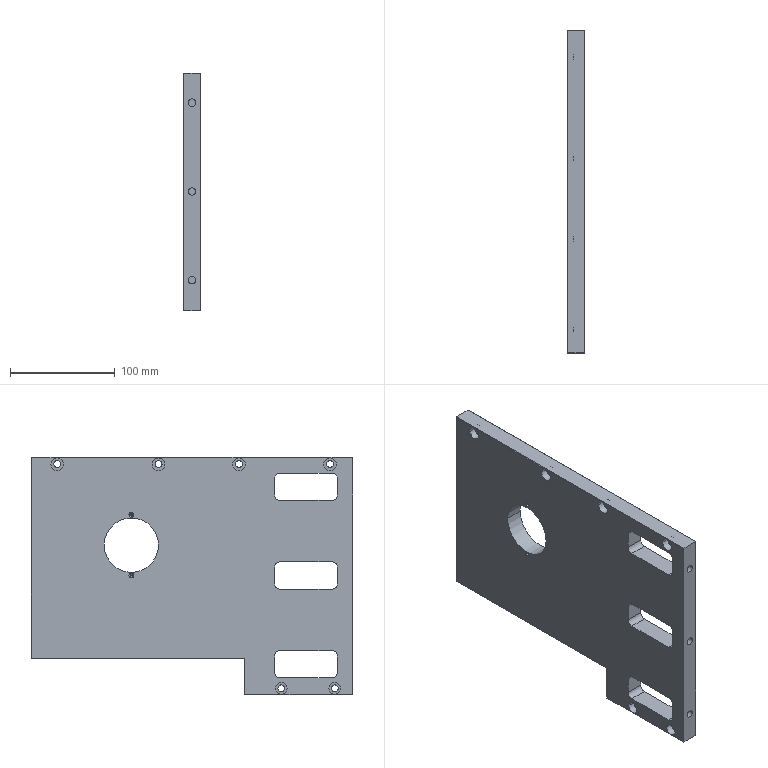Part | NX | 1 solid | 127 faces | box 17 x 308 x 227 mm | volume 942606 mm3 | cylinder 62 | plane 33 | cone 32 | commonest cylinder face diameters 6.6 x12 10 x12 3.3 x10 12 x8 4.2 x6 7 x6